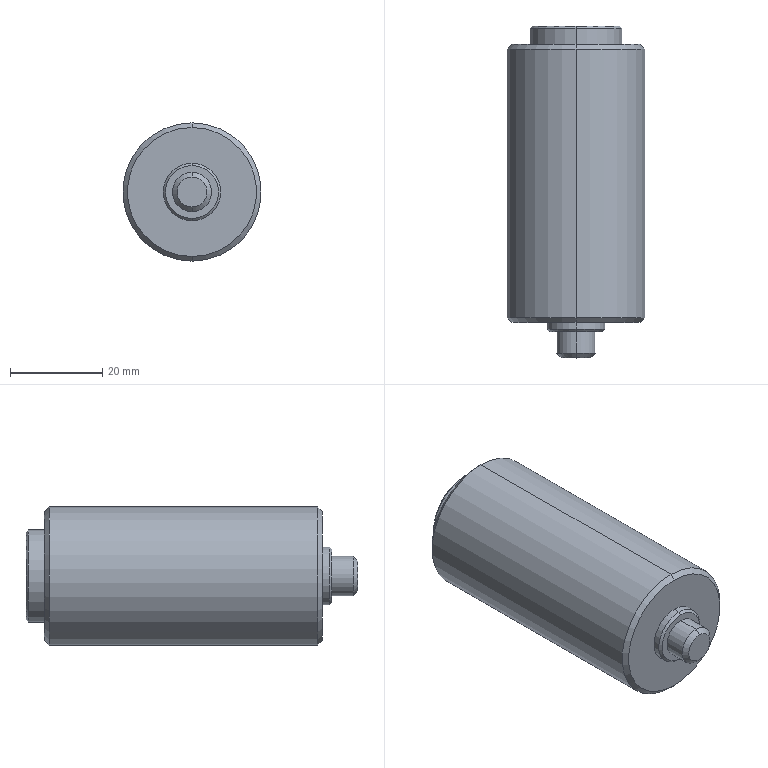Part | SolidWorks | features Chamfer 2, Revolution 1 | 1 solid | 23 faces | box 30 x 72 x 30 mm | volume 44332 mm3 | cone 10 | cylinder 8 | plane 5 | commonest cylinder face diameters 8.5 x2 12.5 x2 20 x2 30 x2
STEP:
#1=CARTESIAN_POINT('',(471.667,-1174.871,-5.75));
#2=VERTEX_POINT('',#1);
#3=CARTESIAN_POINT('',(471.667,-1174.871,5.75));
#4=VERTEX_POINT('',#3);
#5=CARTESIAN_POINT('',(471.667,-1174.871,0.));
#6=DIRECTION('',(0.,-1.,0.));
#7=DIRECTION('',(0.,0.,-1.));
#8=AXIS2_PLACEMENT_3D('',#5,#6,#7);
#9=CIRCLE('',#8,5.75);
#10=EDGE_CURVE('',#2,#4,#9,.T.);
#11=ORIENTED_EDGE('',*,*,#10,.F.);
#12=CARTESIAN_POINT('',(471.667,-1174.371,-6.25));
#13=VERTEX_POINT('',#12);
#14=CARTESIAN_POINT('',(471.667,-1174.871,-5.75));
#15=DIRECTION('',(0.,0.7071,-0.7071));
#16=VECTOR('',#15,1000.);
#17=LINE('',#14,#16);
#18=EDGE_CURVE('',#2,#13,#17,.T.);
#19=ORIENTED_EDGE('',*,*,#18,.T.);
#20=CARTESIAN_POINT('',(471.667,-1174.371,6.25));
#21=VERTEX_POINT('',#20);
#22=CARTESIAN_POINT('',(471.667,-1174.371,0.));
#23=DIRECTION('',(0.,1.,0.));
#24=DIRECTION('',(0.,0.,-1.));
#25=AXIS2_PLACEMENT_3D('',#22,#23,#24);
#26=CIRCLE('',#25,6.25);
#27=EDGE_CURVE('',#21,#13,#26,.T.);
#28=ORIENTED_EDGE('',*,*,#27,.F.);
#29=CARTESIAN_POINT('',(471.667,-1174.871,5.75));
#30=DIRECTION('',(0.,0.7071,0.7071));
#31=VECTOR('',#30,1000.);
#32=LINE('',#29,#31);
#33=EDGE_CURVE('',#4,#21,#32,.T.);
#34=ORIENTED_EDGE('',*,*,#33,.F.);
#35=EDGE_LOOP('',(#11,#19,#28,#34));
#36=FACE_OUTER_BOUND('',#35,.T.);
#37=CARTESIAN_POINT('',(471.667,-1174.871,0.));
#38=DIRECTION('',(0.,1.,0.));
#39=DIRECTION('',(0.,0.,1.));
#40=AXIS2_PLACEMENT_3D('',#37,#38,#39);
#41=CONICAL_SURFACE('',#40,5.75,0.7854);
#42=ADVANCED_FACE('',(#36),#41,.T.);
#43=CARTESIAN_POINT('',(471.667,-1108.571,9.5));
#44=VERTEX_POINT('',#43);
#45=CARTESIAN_POINT('',(471.667,-1108.571,-9.5));
#46=VERTEX_POINT('',#45);
#47=CARTESIAN_POINT('',(471.667,-1108.571,0.));
#48=DIRECTION('',(0.,1.,0.));
#49=DIRECTION('',(0.,0.,1.));
#50=AXIS2_PLACEMENT_3D('',#47,#48,#49);
#51=CIRCLE('',#50,9.5);
#52=EDGE_CURVE('',#44,#46,#51,.T.);
#53=ORIENTED_EDGE('',*,*,#52,.F.);
#54=CARTESIAN_POINT('',(471.667,-1109.071,10.));
#55=VERTEX_POINT('',#54);
#56=CARTESIAN_POINT('',(471.667,-1109.071,10.));
#57=DIRECTION('',(0.,-0.7071,0.7071));
#58=VECTOR('',#57,1000.);
#59=LINE('',#56,#58);
#60=EDGE_CURVE('',#44,#55,#59,.T.);
#61=ORIENTED_EDGE('',*,*,#60,.T.);
#62=CARTESIAN_POINT('',(471.667,-1109.071,-10.));
#63=VERTEX_POINT('',#62);
#64=CARTESIAN_POINT('',(471.667,-1109.071,0.));
#65=DIRECTION('',(0.,-1.,0.));
#66=DIRECTION('',(0.,0.,1.));
#67=AXIS2_PLACEMENT_3D('',#64,#65,#66);
#68=CIRCLE('',#67,10.);
#69=EDGE_CURVE('',#63,#55,#68,.T.);
#70=ORIENTED_EDGE('',*,*,#69,.F.);
#71=CARTESIAN_POINT('',(471.667,-1109.071,-10.));
#72=DIRECTION('',(0.,-0.7071,-0.7071));
#73=VECTOR('',#72,1000.);
#74=LINE('',#71,#73);
#75=EDGE_CURVE('',#46,#63,#74,.T.);
#76=ORIENTED_EDGE('',*,*,#75,.F.);
#77=EDGE_LOOP('',(#53,#61,#70,#76));
#78=FACE_OUTER_BOUND('',#77,.T.);
#79=CARTESIAN_POINT('',(471.667,-1109.071,0.));
#80=DIRECTION('',(0.,-1.,0.));
#81=DIRECTION('',(0.,0.,-1.));
#82=AXIS2_PLACEMENT_3D('',#79,#80,#81);
#83=CONICAL_SURFACE('',#82,10.,0.7854);
#84=ADVANCED_FACE('',(#78),#83,.T.);
#85=CARTESIAN_POINT('',(471.667,-1180.571,-3.25));
#86=VERTEX_POINT('',#85);
#87=CARTESIAN_POINT('',(471.667,-1180.571,3.25));
#88=VERTEX_POINT('',#87);
#89=CARTESIAN_POINT('',(471.667,-1180.571,0.));
#90=DIRECTION('',(0.,-1.,0.));
#91=DIRECTION('',(0.,0.,-1.));
#92=AXIS2_PLACEMENT_3D('',#89,#90,#91);
#93=CIRCLE('',#92,3.25);
#94=EDGE_CURVE('',#86,#88,#93,.T.);
#95=ORIENTED_EDGE('',*,*,#94,.F.);
#96=CARTESIAN_POINT('',(471.667,-1179.571,-4.25));
#97=VERTEX_POINT('',#96);
#98=CARTESIAN_POINT('',(471.667,-1180.571,-3.25));
#99=DIRECTION('',(0.,0.7071,-0.7071));
#100=VECTOR('',#99,1000.);
#101=LINE('',#98,#100);
#102=EDGE_CURVE('',#86,#97,#101,.T.);
#103=ORIENTED_EDGE('',*,*,#102,.T.);
#104=CARTESIAN_POINT('',(471.667,-1179.571,4.25));
#105=VERTEX_POINT('',#104);
#106=CARTESIAN_POINT('',(471.667,-1179.571,0.));
#107=DIRECTION('',(0.,1.,0.));
#108=DIRECTION('',(0.,0.,-1.));
#109=AXIS2_PLACEMENT_3D('',#106,#107,#108);
#110=CIRCLE('',#109,4.25);
#111=EDGE_CURVE('',#105,#97,#110,.T.);
#112=ORIENTED_EDGE('',*,*,#111,.F.);
#113=CARTESIAN_POINT('',(471.667,-1180.571,3.25));
#114=DIRECTION('',(0.,0.7071,0.7071));
#115=VECTOR('',#114,1000.);
#116=LINE('',#113,#115);
#117=EDGE_CURVE('',#88,#105,#116,.T.);
#118=ORIENTED_EDGE('',*,*,#117,.F.);
#119=EDGE_LOOP('',(#95,#103,#112,#118));
#120=FACE_OUTER_BOUND('',#119,.T.);
#121=CARTESIAN_POINT('',(471.667,-1180.571,0.));
#122=DIRECTION('',(0.,1.,0.));
#123=DIRECTION('',(0.,0.,1.));
#124=AXIS2_PLACEMENT_3D('',#121,#122,#123);
#125=CONICAL_SURFACE('',#124,3.25,0.7854);
#126=ADVANCED_FACE('',(#120),#125,.T.);
#127=CARTESIAN_POINT('',(471.667,-1172.871,-14.));
#128=VERTEX_POINT('',#127);
#129=CARTESIAN_POINT('',(471.667,-1172.871,14.));
#130=VERTEX_POINT('',#129);
#131=CARTESIAN_POINT('',(471.667,-1172.871,0.));
#132=DIRECTION('',(0.,-1.,0.));
#133=DIRECTION('',(0.,0.,-1.));
#134=AXIS2_PLACEMENT_3D('',#131,#132,#133);
#135=CIRCLE('',#134,14.);
#136=EDGE_CURVE('',#128,#130,#135,.T.);
#137=ORIENTED_EDGE('',*,*,#136,.F.);
#138=CARTESIAN_POINT('',(471.667,-1171.871,-15.));
#139=VERTEX_POINT('',#138);
#140=CARTESIAN_POINT('',(471.667,-1172.871,-14.));
#141=DIRECTION('',(0.,0.7071,-0.7071));
#142=VECTOR('',#141,1000.);
#143=LINE('',#140,#142);
#144=EDGE_CURVE('',#128,#139,#143,.T.);
#145=ORIENTED_EDGE('',*,*,#144,.T.);
#146=CARTESIAN_POINT('',(471.667,-1171.871,15.));
#147=VERTEX_POINT('',#146);
#148=CARTESIAN_POINT('',(471.667,-1171.871,0.));
#149=DIRECTION('',(0.,1.,0.));
#150=DIRECTION('',(0.,0.,-1.));
#151=AXIS2_PLACEMENT_3D('',#148,#149,#150);
#152=CIRCLE('',#151,15.);
#153=EDGE_CURVE('',#147,#139,#152,.T.);
#154=ORIENTED_EDGE('',*,*,#153,.F.);
#155=CARTESIAN_POINT('',(471.667,-1172.871,14.));
#156=DIRECTION('',(0.,0.7071,0.7071));
#157=VECTOR('',#156,1000.);
#158=LINE('',#155,#157);
#159=EDGE_CURVE('',#130,#147,#158,.T.);
#160=ORIENTED_EDGE('',*,*,#159,.F.);
#161=EDGE_LOOP('',(#137,#145,#154,#160));
#162=FACE_OUTER_BOUND('',#161,.T.);
#163=CARTESIAN_POINT('',(471.667,-1172.871,0.));
#164=DIRECTION('',(0.,1.,0.));
#165=DIRECTION('',(0.,0.,1.));
#166=AXIS2_PLACEMENT_3D('',#163,#164,#165);
#167=CONICAL_SURFACE('',#166,14.,0.7854);
#168=ADVANCED_FACE('',(#162),#167,.T.);
#169=CARTESIAN_POINT('',(471.667,-1112.571,14.));
#170=VERTEX_POINT('',#169);
#171=CARTESIAN_POINT('',(471.667,-1112.571,-14.));
#172=VERTEX_POINT('',#171);
#173=CARTESIAN_POINT('',(471.667,-1112.571,0.));
#174=DIRECTION('',(0.,1.,0.));
#175=DIRECTION('',(0.,0.,1.));
#176=AXIS2_PLACEMENT_3D('',#173,#174,#175);
#177=CIRCLE('',#176,14.);
#178=EDGE_CURVE('',#170,#172,#177,.T.);
#179=ORIENTED_EDGE('',*,*,#178,.F.);
#180=CARTESIAN_POINT('',(471.667,-1113.571,15.));
#181=VERTEX_POINT('',#180);
#182=CARTESIAN_POINT('',(471.667,-1113.571,15.));
#183=DIRECTION('',(0.,-0.7071,0.7071));
#184=VECTOR('',#183,1000.);
#185=LINE('',#182,#184);
#186=EDGE_CURVE('',#170,#181,#185,.T.);
#187=ORIENTED_EDGE('',*,*,#186,.T.);
#188=CARTESIAN_POINT('',(471.667,-1113.571,-15.));
#189=VERTEX_POINT('',#188);
#190=CARTESIAN_POINT('',(471.667,-1113.571,0.));
#191=DIRECTION('',(0.,-1.,0.));
#192=DIRECTION('',(0.,0.,1.));
#193=AXIS2_PLACEMENT_3D('',#190,#191,#192);
#194=CIRCLE('',#193,15.);
#195=EDGE_CURVE('',#189,#181,#194,.T.);
#196=ORIENTED_EDGE('',*,*,#195,.F.);
#197=CARTESIAN_POINT('',(471.667,-1113.571,-15.));
#198=DIRECTION('',(0.,-0.7071,-0.7071));
#199=VECTOR('',#198,1000.);
#200=LINE('',#197,#199);
#201=EDGE_CURVE('',#172,#189,#200,.T.);
#202=ORIENTED_EDGE('',*,*,#201,.F.);
#203=EDGE_LOOP('',(#179,#187,#196,#202));
#204=FACE_OUTER_BOUND('',#203,.T.);
#205=CARTESIAN_POINT('',(471.667,-1113.571,0.));
#206=DIRECTION('',(0.,-1.,0.));
#207=DIRECTION('',(0.,0.,-1.));
#208=AXIS2_PLACEMENT_3D('',#205,#206,#207);
#209=CONICAL_SURFACE('',#208,15.,0.7854);
#210=ADVANCED_FACE('',(#204),#209,.T.);
#211=CARTESIAN_POINT('',(471.667,-1172.871,-6.25));
#212=VERTEX_POINT('',#211);
#213=CARTESIAN_POINT('',(471.667,-1172.871,6.25));
#214=VERTEX_POINT('',#213);
#215=CARTESIAN_POINT('',(471.667,-1172.871,0.));
#216=DIRECTION('',(0.,-1.,0.));
#217=DIRECTION('',(0.,0.,-1.));
#218=AXIS2_PLACEMENT_3D('',#215,#216,#217);
#219=CIRCLE('',#218,6.25);
#220=EDGE_CURVE('',#212,#214,#219,.T.);
#221=ORIENTED_EDGE('',*,*,#220,.T.);
#222=CARTESIAN_POINT('',(471.667,-1180.571,6.25));
#223=DIRECTION('',(0.,-1.,0.));
#224=VECTOR('',#223,1000.);
#225=LINE('',#222,#224);
#226=EDGE_CURVE('',#214,#21,#225,.T.);
#227=ORIENTED_EDGE('',*,*,#226,.T.);
#228=ORIENTED_EDGE('',*,*,#27,.T.);
#229=CARTESIAN_POINT('',(471.667,-1180.571,-6.25));
#230=DIRECTION('',(0.,-1.,0.));
#231=VECTOR('',#230,1000.);
#232=LINE('',#229,#231);
#233=EDGE_CURVE('',#212,#13,#232,.T.);
#234=ORIENTED_EDGE('',*,*,#233,.F.);
#235=EDGE_LOOP('',(#221,#227,#228,#234));
#236=FACE_OUTER_BOUND('',#235,.T.);
#237=CARTESIAN_POINT('',(471.667,-1180.571,0.));
#238=DIRECTION('',(0.,-1.,0.));
#239=DIRECTION('',(0.,0.,-1.));
#240=AXIS2_PLACEMENT_3D('',#237,#238,#239);
#241=CYLINDRICAL_SURFACE('',#240,6.25);
#242=ADVANCED_FACE('',(#236),#241,.T.);
#243=CARTESIAN_POINT('',(471.667,-1174.871,-4.25));
#244=VERTEX_POINT('',#243);
#245=CARTESIAN_POINT('',(471.667,-1174.871,4.25));
#246=VERTEX_POINT('',#245);
#247=CARTESIAN_POINT('',(471.667,-1174.871,0.));
#248=DIRECTION('',(0.,-1.,0.));
#249=DIRECTION('',(0.,0.,-1.));
#250=AXIS2_PLACEMENT_3D('',#247,#248,#249);
#251=CIRCLE('',#250,4.25);
#252=EDGE_CURVE('',#244,#246,#251,.T.);
#253=ORIENTED_EDGE('',*,*,#252,.T.);
#254=CARTESIAN_POINT('',(471.667,-1180.571,4.25));
#255=DIRECTION('',(0.,-1.,0.));
#256=VECTOR('',#255,1000.);
#257=LINE('',#254,#256);
#258=EDGE_CURVE('',#246,#105,#257,.T.);
#259=ORIENTED_EDGE('',*,*,#258,.T.);
#260=ORIENTED_EDGE('',*,*,#111,.T.);
#261=CARTESIAN_POINT('',(471.667,-1180.571,-4.25));
#262=DIRECTION('',(0.,-1.,0.));
#263=VECTOR('',#262,1000.);
#264=LINE('',#261,#263);
#265=EDGE_CURVE('',#244,#97,#264,.T.);
#266=ORIENTED_EDGE('',*,*,#265,.F.);
#267=EDGE_LOOP('',(#253,#259,#260,#266));
#268=FACE_OUTER_BOUND('',#267,.T.);
#269=CARTESIAN_POINT('',(471.667,-1180.571,0.));
#270=DIRECTION('',(0.,-1.,0.));
#271=DIRECTION('',(0.,0.,-1.));
#272=AXIS2_PLACEMENT_3D('',#269,#270,#271);
#273=CYLINDRICAL_SURFACE('',#272,4.25);
#274=ADVANCED_FACE('',(#268),#273,.T.);
#275=ORIENTED_EDGE('',*,*,#69,.T.);
#276=CARTESIAN_POINT('',(471.667,-1112.571,10.));
#277=VERTEX_POINT('',#276);
#278=CARTESIAN_POINT('',(471.667,-1180.571,10.));
#279=DIRECTION('',(0.,-1.,0.));
#280=VECTOR('',#279,1000.);
#281=LINE('',#278,#280);
#282=EDGE_CURVE('',#55,#277,#281,.T.);
#283=ORIENTED_EDGE('',*,*,#282,.T.);
#284=CARTESIAN_POINT('',(471.667,-1112.571,-10.));
#285=VERTEX_POINT('',#284);
#286=CARTESIAN_POINT('',(471.667,-1112.571,0.));
#287=DIRECTION('',(0.,-1.,0.));
#288=DIRECTION('',(0.,0.,-1.));
#289=AXIS2_PLACEMENT_3D('',#286,#287,#288);
#290=CIRCLE('',#289,10.);
#291=EDGE_CURVE('',#285,#277,#290,.T.);
#292=ORIENTED_EDGE('',*,*,#291,.F.);
#293=CARTESIAN_POINT('',(471.667,-1180.571,-10.));
#294=DIRECTION('',(0.,-1.,0.));
#295=VECTOR('',#294,1000.);
#296=LINE('',#293,#295);
#297=EDGE_CURVE('',#63,#285,#296,.T.);
#298=ORIENTED_EDGE('',*,*,#297,.F.);
#299=EDGE_LOOP('',(#275,#283,#292,#298));
#300=FACE_OUTER_BOUND('',#299,.T.);
#301=CARTESIAN_POINT('',(471.667,-1180.571,0.));
#302=DIRECTION('',(0.,-1.,0.));
#303=DIRECTION('',(0.,0.,-1.));
#304=AXIS2_PLACEMENT_3D('',#301,#302,#303);
#305=CYLINDRICAL_SURFACE('',#304,10.);
#306=ADVANCED_FACE('',(#300),#305,.T.);
#307=ORIENTED_EDGE('',*,*,#195,.T.);
#308=CARTESIAN_POINT('',(471.667,-1180.571,15.));
#309=DIRECTION('',(0.,-1.,0.));
#310=VECTOR('',#309,1000.);
#311=LINE('',#308,#310);
#312=EDGE_CURVE('',#181,#147,#311,.T.);
#313=ORIENTED_EDGE('',*,*,#312,.T.);
#314=ORIENTED_EDGE('',*,*,#153,.T.);
#315=CARTESIAN_POINT('',(471.667,-1180.571,-15.));
#316=DIRECTION('',(0.,-1.,0.));
#317=VECTOR('',#316,1000.);
#318=LINE('',#315,#317);
#319=EDGE_CURVE('',#189,#139,#318,.T.);
#320=ORIENTED_EDGE('',*,*,#319,.F.);
#321=EDGE_LOOP('',(#307,#313,#314,#320));
#322=FACE_OUTER_BOUND('',#321,.T.);
#323=CARTESIAN_POINT('',(471.667,-1180.571,0.));
#324=DIRECTION('',(0.,-1.,0.));
#325=DIRECTION('',(0.,0.,-1.));
#326=AXIS2_PLACEMENT_3D('',#323,#324,#325);
#327=CYLINDRICAL_SURFACE('',#326,15.);
#328=ADVANCED_FACE('',(#322),#327,.T.);
#329=CARTESIAN_POINT('',(471.667,-1172.871,0.));
#330=DIRECTION('',(0.,-1.,0.));
#331=DIRECTION('',(0.,0.,-1.));
#332=AXIS2_PLACEMENT_3D('',#329,#330,#331);
#333=CIRCLE('',#332,14.);
#334=EDGE_CURVE('',#130,#128,#333,.T.);
#335=ORIENTED_EDGE('',*,*,#334,.T.);
#336=ORIENTED_EDGE('',*,*,#136,.T.);
#337=EDGE_LOOP('',(#335,#336));
#338=FACE_OUTER_BOUND('',#337,.T.);
#339=ORIENTED_EDGE('',*,*,#220,.F.);
#340=CARTESIAN_POINT('',(471.667,-1172.871,0.));
#341=DIRECTION('',(0.,-1.,0.));
#342=DIRECTION('',(0.,0.,-1.));
#343=AXIS2_PLACEMENT_3D('',#340,#341,#342);
#344=CIRCLE('',#343,6.25);
#345=EDGE_CURVE('',#214,#212,#344,.T.);
#346=ORIENTED_EDGE('',*,*,#345,.F.);
#347=EDGE_LOOP('',(#339,#346));
#348=FACE_BOUND('',#347,.T.);
#349=CARTESIAN_POINT('',(486.667,-1172.871,0.));
#350=DIRECTION('',(0.,-1.,0.));
#351=DIRECTION('',(0.,0.,-1.));
#352=AXIS2_PLACEMENT_3D('',#349,#350,#351);
#353=PLANE('',#352);
#354=ADVANCED_FACE('',(#338,#348),#353,.T.);
#355=ORIENTED_EDGE('',*,*,#312,.F.);
#356=CARTESIAN_POINT('',(471.667,-1113.571,0.));
#357=DIRECTION('',(0.,-1.,0.));
#358=DIRECTION('',(0.,0.,1.));
#359=AXIS2_PLACEMENT_3D('',#356,#357,#358);
#360=CIRCLE('',#359,15.);
#361=EDGE_CURVE('',#181,#189,#360,.T.);
#362=ORIENTED_EDGE('',*,*,#361,.T.);
#363=ORIENTED_EDGE('',*,*,#319,.T.);
#364=CARTESIAN_POINT('',(471.667,-1171.871,0.));
#365=DIRECTION('',(0.,1.,0.));
#366=DIRECTION('',(0.,0.,-1.));
#367=AXIS2_PLACEMENT_3D('',#364,#365,#366);
#368=CIRCLE('',#367,15.);
#369=EDGE_CURVE('',#139,#147,#368,.T.);
#370=ORIENTED_EDGE('',*,*,#369,.T.);
#371=EDGE_LOOP('',(#355,#362,#363,#370));
#372=FACE_OUTER_BOUND('',#371,.T.);
#373=CARTESIAN_POINT('',(471.667,-1180.571,0.));
#374=DIRECTION('',(0.,-1.,0.));
#375=DIRECTION('',(0.,0.,-1.));
#376=AXIS2_PLACEMENT_3D('',#373,#374,#375);
#377=CYLINDRICAL_SURFACE('',#376,15.);
#378=ADVANCED_FACE('',(#372),#377,.T.);
#379=CARTESIAN_POINT('',(471.667,-1112.571,0.));
#380=DIRECTION('',(0.,1.,0.));
#381=DIRECTION('',(0.,0.,1.));
#382=AXIS2_PLACEMENT_3D('',#379,#380,#381);
#383=CIRCLE('',#382,14.);
#384=EDGE_CURVE('',#172,#170,#383,.T.);
#385=ORIENTED_EDGE('',*,*,#384,.T.);
#386=ORIENTED_EDGE('',*,*,#178,.T.);
#387=EDGE_LOOP('',(#385,#386));
#388=FACE_OUTER_BOUND('',#387,.T.);
#389=ORIENTED_EDGE('',*,*,#291,.T.);
#390=CARTESIAN_POINT('',(471.667,-1112.571,0.));
#391=DIRECTION('',(0.,-1.,0.));
#392=DIRECTION('',(0.,0.,-1.));
#393=AXIS2_PLACEMENT_3D('',#390,#391,#392);
#394=CIRCLE('',#393,10.);
#395=EDGE_CURVE('',#277,#285,#394,.T.);
#396=ORIENTED_EDGE('',*,*,#395,.T.);
#397=EDGE_LOOP('',(#389,#396));
#398=FACE_BOUND('',#397,.T.);
#399=CARTESIAN_POINT('',(486.667,-1112.571,0.));
#400=DIRECTION('',(0.,1.,0.));
#401=DIRECTION('',(0.,0.,1.));
#402=AXIS2_PLACEMENT_3D('',#399,#400,#401);
#403=PLANE('',#402);
#404=ADVANCED_FACE('',(#388,#398),#403,.T.);
#405=ORIENTED_EDGE('',*,*,#282,.F.);
#406=CARTESIAN_POINT('',(471.667,-1109.071,0.));
#407=DIRECTION('',(0.,-1.,0.));
#408=DIRECTION('',(0.,0.,1.));
#409=AXIS2_PLACEMENT_3D('',#406,#407,#408);
#410=CIRCLE('',#409,10.);
#411=EDGE_CURVE('',#55,#63,#410,.T.);
#412=ORIENTED_EDGE('',*,*,#411,.T.);
#413=ORIENTED_EDGE('',*,*,#297,.T.);
#414=ORIENTED_EDGE('',*,*,#395,.F.);
#415=EDGE_LOOP('',(#405,#412,#413,#414));
#416=FACE_OUTER_BOUND('',#415,.T.);
#417=CARTESIAN_POINT('',(471.667,-1180.571,0.));
#418=DIRECTION('',(0.,-1.,0.));
#419=DIRECTION('',(0.,0.,-1.));
#420=AXIS2_PLACEMENT_3D('',#417,#418,#419);
#421=CYLINDRICAL_SURFACE('',#420,10.);
#422=ADVANCED_FACE('',(#416),#421,.T.);
#423=CARTESIAN_POINT('',(471.667,-1108.571,0.));
#424=DIRECTION('',(0.,1.,0.));
#425=DIRECTION('',(0.,0.,1.));
#426=AXIS2_PLACEMENT_3D('',#423,#424,#425);
#427=CIRCLE('',#426,9.5);
#428=EDGE_CURVE('',#46,#44,#427,.T.);
#429=ORIENTED_EDGE('',*,*,#428,.T.);
#430=ORIENTED_EDGE('',*,*,#52,.T.);
#431=EDGE_LOOP('',(#429,#430));
#432=FACE_OUTER_BOUND('',#431,.T.);
#433=CARTESIAN_POINT('',(481.667,-1108.571,0.));
#434=DIRECTION('',(0.,1.,0.));
#435=DIRECTION('',(0.,0.,1.));
#436=AXIS2_PLACEMENT_3D('',#433,#434,#435);
#437=PLANE('',#436);
#438=ADVANCED_FACE('',(#432),#437,.T.);
#439=CARTESIAN_POINT('',(471.667,-1180.571,0.));
#440=DIRECTION('',(0.,-1.,0.));
#441=DIRECTION('',(0.,0.,-1.));
#442=AXIS2_PLACEMENT_3D('',#439,#440,#441);
#443=CIRCLE('',#442,3.25);
#444=EDGE_CURVE('',#88,#86,#443,.T.);
#445=ORIENTED_EDGE('',*,*,#444,.T.);
#446=ORIENTED_EDGE('',*,*,#94,.T.);
#447=EDGE_LOOP('',(#445,#446));
#448=FACE_OUTER_BOUND('',#447,.T.);
#449=CARTESIAN_POINT('',(475.917,-1180.571,0.));
#450=DIRECTION('',(0.,-1.,0.));
#451=DIRECTION('',(0.,0.,-1.));
#452=AXIS2_PLACEMENT_3D('',#449,#450,#451);
#453=PLANE('',#452);
#454=ADVANCED_FACE('',(#448),#453,.T.);
#455=ORIENTED_EDGE('',*,*,#258,.F.);
#456=CARTESIAN_POINT('',(471.667,-1174.871,0.));
#457=DIRECTION('',(0.,-1.,0.));
#458=DIRECTION('',(0.,0.,-1.));
#459=AXIS2_PLACEMENT_3D('',#456,#457,#458);
#460=CIRCLE('',#459,4.25);
#461=EDGE_CURVE('',#246,#244,#460,.T.);
#462=ORIENTED_EDGE('',*,*,#461,.T.);
#463=ORIENTED_EDGE('',*,*,#265,.T.);
#464=CARTESIAN_POINT('',(471.667,-1179.571,0.));
#465=DIRECTION('',(0.,1.,0.));
#466=DIRECTION('',(0.,0.,-1.));
#467=AXIS2_PLACEMENT_3D('',#464,#465,#466);
#468=CIRCLE('',#467,4.25);
#469=EDGE_CURVE('',#97,#105,#468,.T.);
#470=ORIENTED_EDGE('',*,*,#469,.T.);
#471=EDGE_LOOP('',(#455,#462,#463,#470));
#472=FACE_OUTER_BOUND('',#471,.T.);
#473=CARTESIAN_POINT('',(471.667,-1180.571,0.));
#474=DIRECTION('',(0.,-1.,0.));
#475=DIRECTION('',(0.,0.,-1.));
#476=AXIS2_PLACEMENT_3D('',#473,#474,#475);
#477=CYLINDRICAL_SURFACE('',#476,4.25);
#478=ADVANCED_FACE('',(#472),#477,.T.);
#479=CARTESIAN_POINT('',(471.667,-1174.871,0.));
#480=DIRECTION('',(0.,-1.,0.));
#481=DIRECTION('',(0.,0.,-1.));
#482=AXIS2_PLACEMENT_3D('',#479,#480,#481);
#483=CIRCLE('',#482,5.75);
#484=EDGE_CURVE('',#4,#2,#483,.T.);
#485=ORIENTED_EDGE('',*,*,#484,.T.);
#486=ORIENTED_EDGE('',*,*,#10,.T.);
#487=EDGE_LOOP('',(#485,#486));
#488=FACE_OUTER_BOUND('',#487,.T.);
#489=ORIENTED_EDGE('',*,*,#252,.F.);
#490=ORIENTED_EDGE('',*,*,#461,.F.);
#491=EDGE_LOOP('',(#489,#490));
#492=FACE_BOUND('',#491,.T.);
#493=CARTESIAN_POINT('',(477.917,-1174.871,0.));
#494=DIRECTION('',(0.,-1.,0.));
#495=DIRECTION('',(0.,0.,-1.));
#496=AXIS2_PLACEMENT_3D('',#493,#494,#495);
#497=PLANE('',#496);
#498=ADVANCED_FACE('',(#488,#492),#497,.T.);
#499=ORIENTED_EDGE('',*,*,#226,.F.);
#500=ORIENTED_EDGE('',*,*,#345,.T.);
#501=ORIENTED_EDGE('',*,*,#233,.T.);
#502=CARTESIAN_POINT('',(471.667,-1174.371,0.));
#503=DIRECTION('',(0.,1.,0.));
#504=DIRECTION('',(0.,0.,-1.));
#505=AXIS2_PLACEMENT_3D('',#502,#503,#504);
#506=CIRCLE('',#505,6.25);
#507=EDGE_CURVE('',#13,#21,#506,.T.);
#508=ORIENTED_EDGE('',*,*,#507,.T.);
#509=EDGE_LOOP('',(#499,#500,#501,#508));
#510=FACE_OUTER_BOUND('',#509,.T.);
#511=CARTESIAN_POINT('',(471.667,-1180.571,0.));
#512=DIRECTION('',(0.,-1.,0.));
#513=DIRECTION('',(0.,0.,-1.));
#514=AXIS2_PLACEMENT_3D('',#511,#512,#513);
#515=CYLINDRICAL_SURFACE('',#514,6.25);
#516=ADVANCED_FACE('',(#510),#515,.T.);
#517=ORIENTED_EDGE('',*,*,#186,.F.);
#518=ORIENTED_EDGE('',*,*,#384,.F.);
#519=ORIENTED_EDGE('',*,*,#201,.T.);
#520=ORIENTED_EDGE('',*,*,#361,.F.);
#521=EDGE_LOOP('',(#517,#518,#519,#520));
#522=FACE_OUTER_BOUND('',#521,.T.);
#523=CARTESIAN_POINT('',(471.667,-1113.571,0.));
#524=DIRECTION('',(0.,-1.,0.));
#525=DIRECTION('',(0.,0.,-1.));
#526=AXIS2_PLACEMENT_3D('',#523,#524,#525);
#527=CONICAL_SURFACE('',#526,15.,0.7854);
#528=ADVANCED_FACE('',(#522),#527,.T.);
#529=ORIENTED_EDGE('',*,*,#144,.F.);
#530=ORIENTED_EDGE('',*,*,#334,.F.);
#531=ORIENTED_EDGE('',*,*,#159,.T.);
#532=ORIENTED_EDGE('',*,*,#369,.F.);
#533=EDGE_LOOP('',(#529,#530,#531,#532));
#534=FACE_OUTER_BOUND('',#533,.T.);
#535=CARTESIAN_POINT('',(471.667,-1172.871,0.));
#536=DIRECTION('',(0.,1.,0.));
#537=DIRECTION('',(0.,0.,1.));
#538=AXIS2_PLACEMENT_3D('',#535,#536,#537);
#539=CONICAL_SURFACE('',#538,14.,0.7854);
#540=ADVANCED_FACE('',(#534),#539,.T.);
#541=ORIENTED_EDGE('',*,*,#102,.F.);
#542=ORIENTED_EDGE('',*,*,#444,.F.);
#543=ORIENTED_EDGE('',*,*,#117,.T.);
#544=ORIENTED_EDGE('',*,*,#469,.F.);
#545=EDGE_LOOP('',(#541,#542,#543,#544));
#546=FACE_OUTER_BOUND('',#545,.T.);
#547=CARTESIAN_POINT('',(471.667,-1180.571,0.));
#548=DIRECTION('',(0.,1.,0.));
#549=DIRECTION('',(0.,0.,1.));
#550=AXIS2_PLACEMENT_3D('',#547,#548,#549);
#551=CONICAL_SURFACE('',#550,3.25,0.7854);
#552=ADVANCED_FACE('',(#546),#551,.T.);
#553=ORIENTED_EDGE('',*,*,#60,.F.);
#554=ORIENTED_EDGE('',*,*,#428,.F.);
#555=ORIENTED_EDGE('',*,*,#75,.T.);
#556=ORIENTED_EDGE('',*,*,#411,.F.);
#557=EDGE_LOOP('',(#553,#554,#555,#556));
#558=FACE_OUTER_BOUND('',#557,.T.);
#559=CARTESIAN_POINT('',(471.667,-1109.071,0.));
#560=DIRECTION('',(0.,-1.,0.));
#561=DIRECTION('',(0.,0.,-1.));
#562=AXIS2_PLACEMENT_3D('',#559,#560,#561);
#563=CONICAL_SURFACE('',#562,10.,0.7854);
#564=ADVANCED_FACE('',(#558),#563,.T.);
#565=ORIENTED_EDGE('',*,*,#18,.F.);
#566=ORIENTED_EDGE('',*,*,#484,.F.);
#567=ORIENTED_EDGE('',*,*,#33,.T.);
#568=ORIENTED_EDGE('',*,*,#507,.F.);
#569=EDGE_LOOP('',(#565,#566,#567,#568));
#570=FACE_OUTER_BOUND('',#569,.T.);
#571=CARTESIAN_POINT('',(471.667,-1174.871,0.));
#572=DIRECTION('',(0.,1.,0.));
#573=DIRECTION('',(0.,0.,1.));
#574=AXIS2_PLACEMENT_3D('',#571,#572,#573);
#575=CONICAL_SURFACE('',#574,5.75,0.7854);
#576=ADVANCED_FACE('',(#570),#575,.T.);
#577=CLOSED_SHELL('',(#42,#84,#126,#168,#210,#242,#274,#306,#328,#354,#378,#404,#422,#438,#454,#478,#498,#516,#528,#540,#552,#564,#576));
#578=MANIFOLD_SOLID_BREP('',#577);
#579=CARTESIAN_POINT('',(0.,0.,0.));
#580=DIRECTION('',(0.,0.,1.));
#581=DIRECTION('',(1.,0.,0.));
#582=AXIS2_PLACEMENT_3D('',#579,#580,#581);
#583=(LENGTH_UNIT()NAMED_UNIT(*)SI_UNIT(.MILLI.,.METRE.));
#584=UNCERTAINTY_MEASURE_WITH_UNIT(LENGTH_MEASURE(0.00001),#583,'','');
#585=(NAMED_UNIT(*)PLANE_ANGLE_UNIT()SI_UNIT($,.RADIAN.));
#586=(NAMED_UNIT(*)SI_UNIT($,.STERADIAN.)SOLID_ANGLE_UNIT());
#587=(GEOMETRIC_REPRESENTATION_CONTEXT(3)GLOBAL_UNCERTAINTY_ASSIGNED_CONTEXT((#584))GLOBAL_UNIT_ASSIGNED_CONTEXT((#583,#585,#586))REPRESENTATION_CONTEXT('',''));
#588=ADVANCED_BREP_SHAPE_REPRESENTATION('',(#578,#582),#587);